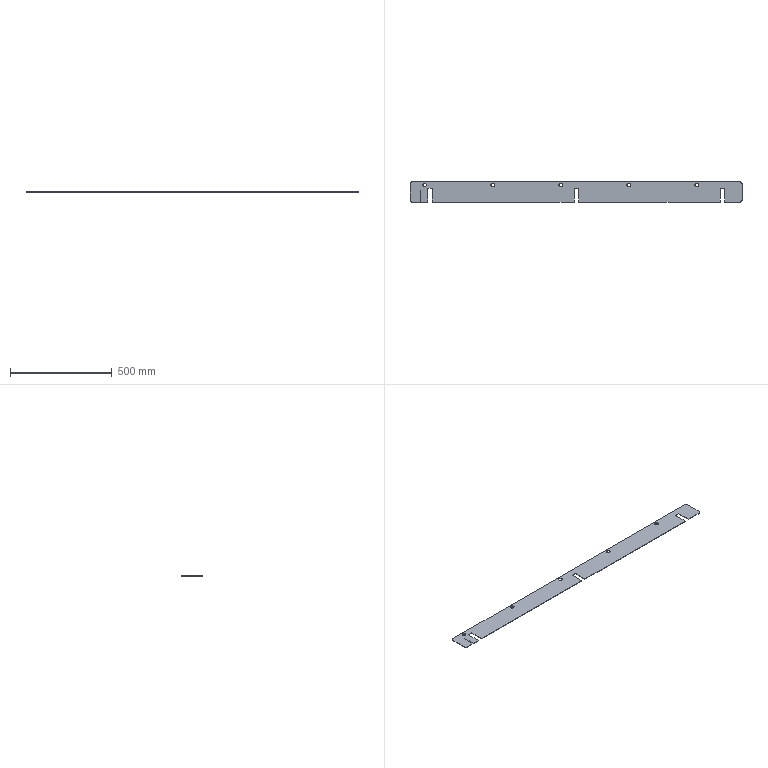Part | SolidWorks | features FlatPattern 1, SMBaseFlange 1, SheetMetal 1 | 1 solid | 36 faces | box 1635 x 100 x 2.3 mm | volume 362359 mm3 | plane 22 | cylinder 14 | commonest cylinder face diameters 18 x10 20 x4
STEP:
#1=CARTESIAN_POINT('',(398.,53.917,2.3));
#2=VERTEX_POINT('',#1);
#3=CARTESIAN_POINT('',(416.,53.917,2.3));
#4=VERTEX_POINT('',#3);
#5=CARTESIAN_POINT('',(407.,53.917,2.3));
#6=DIRECTION('',(0.,0.,1.));
#7=DIRECTION('',(1.,0.,0.));
#8=AXIS2_PLACEMENT_3D('',#5,#6,#7);
#9=CIRCLE('',#8,9.);
#10=EDGE_CURVE('',#2,#4,#9,.T.);
#11=ORIENTED_EDGE('',*,*,#10,.T.);
#12=CARTESIAN_POINT('',(416.,53.917,0.));
#13=VERTEX_POINT('',#12);
#14=CARTESIAN_POINT('',(416.,53.917,2.3));
#15=DIRECTION('',(0.,0.,-1.));
#16=VECTOR('',#15,1000.);
#17=LINE('',#14,#16);
#18=EDGE_CURVE('',#4,#13,#17,.T.);
#19=ORIENTED_EDGE('',*,*,#18,.T.);
#20=CARTESIAN_POINT('',(398.,53.917,0.));
#21=VERTEX_POINT('',#20);
#22=CARTESIAN_POINT('',(407.,53.917,0.));
#23=DIRECTION('',(0.,0.,1.));
#24=DIRECTION('',(1.,0.,0.));
#25=AXIS2_PLACEMENT_3D('',#22,#23,#24);
#26=CIRCLE('',#25,9.);
#27=EDGE_CURVE('',#21,#13,#26,.T.);
#28=ORIENTED_EDGE('',*,*,#27,.F.);
#29=CARTESIAN_POINT('',(398.,53.917,2.3));
#30=DIRECTION('',(0.,0.,-1.));
#31=VECTOR('',#30,1000.);
#32=LINE('',#29,#31);
#33=EDGE_CURVE('',#2,#21,#32,.T.);
#34=ORIENTED_EDGE('',*,*,#33,.F.);
#35=EDGE_LOOP('',(#11,#19,#28,#34));
#36=FACE_OUTER_BOUND('',#35,.T.);
#37=CARTESIAN_POINT('',(407.,53.917,2.3));
#38=DIRECTION('',(0.,0.,-1.));
#39=DIRECTION('',(-1.,0.,0.));
#40=AXIS2_PLACEMENT_3D('',#37,#38,#39);
#41=CYLINDRICAL_SURFACE('',#40,9.);
#42=ADVANCED_FACE('',(#36),#41,.F.);
#43=CARTESIAN_POINT('',(733.,53.917,2.3));
#44=VERTEX_POINT('',#43);
#45=CARTESIAN_POINT('',(751.,53.917,2.3));
#46=VERTEX_POINT('',#45);
#47=CARTESIAN_POINT('',(742.,53.917,2.3));
#48=DIRECTION('',(0.,0.,1.));
#49=DIRECTION('',(1.,0.,0.));
#50=AXIS2_PLACEMENT_3D('',#47,#48,#49);
#51=CIRCLE('',#50,9.);
#52=EDGE_CURVE('',#44,#46,#51,.T.);
#53=ORIENTED_EDGE('',*,*,#52,.T.);
#54=CARTESIAN_POINT('',(751.,53.917,0.));
#55=VERTEX_POINT('',#54);
#56=CARTESIAN_POINT('',(751.,53.917,2.3));
#57=DIRECTION('',(0.,0.,-1.));
#58=VECTOR('',#57,1000.);
#59=LINE('',#56,#58);
#60=EDGE_CURVE('',#46,#55,#59,.T.);
#61=ORIENTED_EDGE('',*,*,#60,.T.);
#62=CARTESIAN_POINT('',(733.,53.917,0.));
#63=VERTEX_POINT('',#62);
#64=CARTESIAN_POINT('',(742.,53.917,0.));
#65=DIRECTION('',(0.,0.,1.));
#66=DIRECTION('',(1.,0.,0.));
#67=AXIS2_PLACEMENT_3D('',#64,#65,#66);
#68=CIRCLE('',#67,9.);
#69=EDGE_CURVE('',#63,#55,#68,.T.);
#70=ORIENTED_EDGE('',*,*,#69,.F.);
#71=CARTESIAN_POINT('',(733.,53.917,2.3));
#72=DIRECTION('',(0.,0.,-1.));
#73=VECTOR('',#72,1000.);
#74=LINE('',#71,#73);
#75=EDGE_CURVE('',#44,#63,#74,.T.);
#76=ORIENTED_EDGE('',*,*,#75,.F.);
#77=EDGE_LOOP('',(#53,#61,#70,#76));
#78=FACE_OUTER_BOUND('',#77,.T.);
#79=CARTESIAN_POINT('',(742.,53.917,2.3));
#80=DIRECTION('',(0.,0.,-1.));
#81=DIRECTION('',(-1.,0.,0.));
#82=AXIS2_PLACEMENT_3D('',#79,#80,#81);
#83=CYLINDRICAL_SURFACE('',#82,9.);
#84=ADVANCED_FACE('',(#78),#83,.F.);
#85=CARTESIAN_POINT('',(1068.,53.917,2.3));
#86=VERTEX_POINT('',#85);
#87=CARTESIAN_POINT('',(1086.,53.917,2.3));
#88=VERTEX_POINT('',#87);
#89=CARTESIAN_POINT('',(1077.,53.917,2.3));
#90=DIRECTION('',(0.,0.,1.));
#91=DIRECTION('',(1.,0.,0.));
#92=AXIS2_PLACEMENT_3D('',#89,#90,#91);
#93=CIRCLE('',#92,9.);
#94=EDGE_CURVE('',#86,#88,#93,.T.);
#95=ORIENTED_EDGE('',*,*,#94,.T.);
#96=CARTESIAN_POINT('',(1086.,53.917,0.));
#97=VERTEX_POINT('',#96);
#98=CARTESIAN_POINT('',(1086.,53.917,2.3));
#99=DIRECTION('',(0.,0.,-1.));
#100=VECTOR('',#99,1000.);
#101=LINE('',#98,#100);
#102=EDGE_CURVE('',#88,#97,#101,.T.);
#103=ORIENTED_EDGE('',*,*,#102,.T.);
#104=CARTESIAN_POINT('',(1068.,53.917,0.));
#105=VERTEX_POINT('',#104);
#106=CARTESIAN_POINT('',(1077.,53.917,0.));
#107=DIRECTION('',(0.,0.,1.));
#108=DIRECTION('',(1.,0.,0.));
#109=AXIS2_PLACEMENT_3D('',#106,#107,#108);
#110=CIRCLE('',#109,9.);
#111=EDGE_CURVE('',#105,#97,#110,.T.);
#112=ORIENTED_EDGE('',*,*,#111,.F.);
#113=CARTESIAN_POINT('',(1068.,53.917,2.3));
#114=DIRECTION('',(0.,0.,-1.));
#115=VECTOR('',#114,1000.);
#116=LINE('',#113,#115);
#117=EDGE_CURVE('',#86,#105,#116,.T.);
#118=ORIENTED_EDGE('',*,*,#117,.F.);
#119=EDGE_LOOP('',(#95,#103,#112,#118));
#120=FACE_OUTER_BOUND('',#119,.T.);
#121=CARTESIAN_POINT('',(1077.,53.917,2.3));
#122=DIRECTION('',(0.,0.,-1.));
#123=DIRECTION('',(-1.,0.,0.));
#124=AXIS2_PLACEMENT_3D('',#121,#122,#123);
#125=CYLINDRICAL_SURFACE('',#124,9.);
#126=ADVANCED_FACE('',(#120),#125,.F.);
#127=CARTESIAN_POINT('',(63.,53.917,2.3));
#128=VERTEX_POINT('',#127);
#129=CARTESIAN_POINT('',(81.,53.917,2.3));
#130=VERTEX_POINT('',#129);
#131=CARTESIAN_POINT('',(72.,53.917,2.3));
#132=DIRECTION('',(0.,0.,1.));
#133=DIRECTION('',(1.,0.,0.));
#134=AXIS2_PLACEMENT_3D('',#131,#132,#133);
#135=CIRCLE('',#134,9.);
#136=EDGE_CURVE('',#128,#130,#135,.T.);
#137=ORIENTED_EDGE('',*,*,#136,.T.);
#138=CARTESIAN_POINT('',(81.,53.917,0.));
#139=VERTEX_POINT('',#138);
#140=CARTESIAN_POINT('',(81.,53.917,2.3));
#141=DIRECTION('',(0.,0.,-1.));
#142=VECTOR('',#141,1000.);
#143=LINE('',#140,#142);
#144=EDGE_CURVE('',#130,#139,#143,.T.);
#145=ORIENTED_EDGE('',*,*,#144,.T.);
#146=CARTESIAN_POINT('',(63.,53.917,0.));
#147=VERTEX_POINT('',#146);
#148=CARTESIAN_POINT('',(72.,53.917,0.));
#149=DIRECTION('',(0.,0.,1.));
#150=DIRECTION('',(1.,0.,0.));
#151=AXIS2_PLACEMENT_3D('',#148,#149,#150);
#152=CIRCLE('',#151,9.);
#153=EDGE_CURVE('',#147,#139,#152,.T.);
#154=ORIENTED_EDGE('',*,*,#153,.F.);
#155=CARTESIAN_POINT('',(63.,53.917,2.3));
#156=DIRECTION('',(0.,0.,-1.));
#157=VECTOR('',#156,1000.);
#158=LINE('',#155,#157);
#159=EDGE_CURVE('',#128,#147,#158,.T.);
#160=ORIENTED_EDGE('',*,*,#159,.F.);
#161=EDGE_LOOP('',(#137,#145,#154,#160));
#162=FACE_OUTER_BOUND('',#161,.T.);
#163=CARTESIAN_POINT('',(72.,53.917,2.3));
#164=DIRECTION('',(0.,0.,-1.));
#165=DIRECTION('',(-1.,0.,0.));
#166=AXIS2_PLACEMENT_3D('',#163,#164,#165);
#167=CYLINDRICAL_SURFACE('',#166,9.);
#168=ADVANCED_FACE('',(#162),#167,.F.);
#169=CARTESIAN_POINT('',(1403.,53.917,2.3));
#170=VERTEX_POINT('',#169);
#171=CARTESIAN_POINT('',(1421.,53.917,2.3));
#172=VERTEX_POINT('',#171);
#173=CARTESIAN_POINT('',(1412.,53.917,2.3));
#174=DIRECTION('',(0.,0.,1.));
#175=DIRECTION('',(1.,0.,0.));
#176=AXIS2_PLACEMENT_3D('',#173,#174,#175);
#177=CIRCLE('',#176,9.);
#178=EDGE_CURVE('',#170,#172,#177,.T.);
#179=ORIENTED_EDGE('',*,*,#178,.T.);
#180=CARTESIAN_POINT('',(1421.,53.917,0.));
#181=VERTEX_POINT('',#180);
#182=CARTESIAN_POINT('',(1421.,53.917,2.3));
#183=DIRECTION('',(0.,0.,-1.));
#184=VECTOR('',#183,1000.);
#185=LINE('',#182,#184);
#186=EDGE_CURVE('',#172,#181,#185,.T.);
#187=ORIENTED_EDGE('',*,*,#186,.T.);
#188=CARTESIAN_POINT('',(1403.,53.917,0.));
#189=VERTEX_POINT('',#188);
#190=CARTESIAN_POINT('',(1412.,53.917,0.));
#191=DIRECTION('',(0.,0.,1.));
#192=DIRECTION('',(1.,0.,0.));
#193=AXIS2_PLACEMENT_3D('',#190,#191,#192);
#194=CIRCLE('',#193,9.);
#195=EDGE_CURVE('',#189,#181,#194,.T.);
#196=ORIENTED_EDGE('',*,*,#195,.F.);
#197=CARTESIAN_POINT('',(1403.,53.917,2.3));
#198=DIRECTION('',(0.,0.,-1.));
#199=VECTOR('',#198,1000.);
#200=LINE('',#197,#199);
#201=EDGE_CURVE('',#170,#189,#200,.T.);
#202=ORIENTED_EDGE('',*,*,#201,.F.);
#203=EDGE_LOOP('',(#179,#187,#196,#202));
#204=FACE_OUTER_BOUND('',#203,.T.);
#205=CARTESIAN_POINT('',(1412.,53.917,2.3));
#206=DIRECTION('',(0.,0.,-1.));
#207=DIRECTION('',(-1.,0.,0.));
#208=AXIS2_PLACEMENT_3D('',#205,#206,#207);
#209=CYLINDRICAL_SURFACE('',#208,9.);
#210=ADVANCED_FACE('',(#204),#209,.F.);
#211=CARTESIAN_POINT('',(88.,38.092,2.3));
#212=VERTEX_POINT('',#211);
#213=CARTESIAN_POINT('',(110.,38.092,2.3));
#214=VERTEX_POINT('',#213);
#215=CARTESIAN_POINT('',(88.,38.092,2.3));
#216=DIRECTION('',(1.,0.,0.));
#217=VECTOR('',#216,1000.);
#218=LINE('',#215,#217);
#219=EDGE_CURVE('',#212,#214,#218,.T.);
#220=ORIENTED_EDGE('',*,*,#219,.T.);
#221=CARTESIAN_POINT('',(110.,-30.083,2.3));
#222=VERTEX_POINT('',#221);
#223=CARTESIAN_POINT('',(110.,38.092,2.3));
#224=DIRECTION('',(0.,-1.,0.));
#225=VECTOR('',#224,1000.);
#226=LINE('',#223,#225);
#227=EDGE_CURVE('',#214,#222,#226,.T.);
#228=ORIENTED_EDGE('',*,*,#227,.T.);
#229=CARTESIAN_POINT('',(808.,-30.083,2.3));
#230=VERTEX_POINT('',#229);
#231=CARTESIAN_POINT('',(110.,-30.083,2.3));
#232=DIRECTION('',(1.,0.,0.));
#233=VECTOR('',#232,1000.);
#234=LINE('',#231,#233);
#235=EDGE_CURVE('',#222,#230,#234,.T.);
#236=ORIENTED_EDGE('',*,*,#235,.T.);
#237=CARTESIAN_POINT('',(808.,38.092,2.3));
#238=VERTEX_POINT('',#237);
#239=CARTESIAN_POINT('',(808.,-30.083,2.3));
#240=DIRECTION('',(0.,1.,0.));
#241=VECTOR('',#240,1000.);
#242=LINE('',#239,#241);
#243=EDGE_CURVE('',#230,#238,#242,.T.);
#244=ORIENTED_EDGE('',*,*,#243,.T.);
#245=CARTESIAN_POINT('',(830.,38.092,2.3));
#246=VERTEX_POINT('',#245);
#247=CARTESIAN_POINT('',(808.,38.092,2.3));
#248=DIRECTION('',(1.,0.,0.));
#249=VECTOR('',#248,1000.);
#250=LINE('',#247,#249);
#251=EDGE_CURVE('',#238,#246,#250,.T.);
#252=ORIENTED_EDGE('',*,*,#251,.T.);
#253=CARTESIAN_POINT('',(830.,-30.083,2.3));
#254=VERTEX_POINT('',#253);
#255=CARTESIAN_POINT('',(830.,38.092,2.3));
#256=DIRECTION('',(0.,-1.,0.));
#257=VECTOR('',#256,1000.);
#258=LINE('',#255,#257);
#259=EDGE_CURVE('',#246,#254,#258,.T.);
#260=ORIENTED_EDGE('',*,*,#259,.T.);
#261=CARTESIAN_POINT('',(1528.,-30.083,2.3));
#262=VERTEX_POINT('',#261);
#263=CARTESIAN_POINT('',(830.,-30.083,2.3));
#264=DIRECTION('',(1.,0.,0.));
#265=VECTOR('',#264,1000.);
#266=LINE('',#263,#265);
#267=EDGE_CURVE('',#254,#262,#266,.T.);
#268=ORIENTED_EDGE('',*,*,#267,.T.);
#269=CARTESIAN_POINT('',(1528.,38.092,2.3));
#270=VERTEX_POINT('',#269);
#271=CARTESIAN_POINT('',(1528.,-30.083,2.3));
#272=DIRECTION('',(0.,1.,0.));
#273=VECTOR('',#272,1000.);
#274=LINE('',#271,#273);
#275=EDGE_CURVE('',#262,#270,#274,.T.);
#276=ORIENTED_EDGE('',*,*,#275,.T.);
#277=CARTESIAN_POINT('',(1550.,38.092,2.3));
#278=VERTEX_POINT('',#277);
#279=CARTESIAN_POINT('',(1528.,38.092,2.3));
#280=DIRECTION('',(1.,0.,0.));
#281=VECTOR('',#280,1000.);
#282=LINE('',#279,#281);
#283=EDGE_CURVE('',#270,#278,#282,.T.);
#284=ORIENTED_EDGE('',*,*,#283,.T.);
#285=CARTESIAN_POINT('',(1550.,-30.083,2.3));
#286=VERTEX_POINT('',#285);
#287=CARTESIAN_POINT('',(1550.,38.092,2.3));
#288=DIRECTION('',(0.,-1.,0.));
#289=VECTOR('',#288,1000.);
#290=LINE('',#287,#289);
#291=EDGE_CURVE('',#278,#286,#290,.T.);
#292=ORIENTED_EDGE('',*,*,#291,.T.);
#293=CARTESIAN_POINT('',(1625.,-30.083,2.3));
#294=VERTEX_POINT('',#293);
#295=CARTESIAN_POINT('',(1550.,-30.083,2.3));
#296=DIRECTION('',(1.,0.,0.));
#297=VECTOR('',#296,1000.);
#298=LINE('',#295,#297);
#299=EDGE_CURVE('',#286,#294,#298,.T.);
#300=ORIENTED_EDGE('',*,*,#299,.T.);
#301=CARTESIAN_POINT('',(1635.,-20.083,2.3));
#302=VERTEX_POINT('',#301);
#303=CARTESIAN_POINT('',(1625.,-20.083,2.3));
#304=DIRECTION('',(0.,0.,1.));
#305=DIRECTION('',(-1.,0.,0.));
#306=AXIS2_PLACEMENT_3D('',#303,#304,#305);
#307=CIRCLE('',#306,10.);
#308=EDGE_CURVE('',#294,#302,#307,.T.);
#309=ORIENTED_EDGE('',*,*,#308,.T.);
#310=CARTESIAN_POINT('',(1635.,59.917,2.3));
#311=VERTEX_POINT('',#310);
#312=CARTESIAN_POINT('',(1635.,-20.083,2.3));
#313=DIRECTION('',(0.,1.,0.));
#314=VECTOR('',#313,1000.);
#315=LINE('',#312,#314);
#316=EDGE_CURVE('',#302,#311,#315,.T.);
#317=ORIENTED_EDGE('',*,*,#316,.T.);
#318=CARTESIAN_POINT('',(1625.,69.917,2.3));
#319=VERTEX_POINT('',#318);
#320=CARTESIAN_POINT('',(1625.,59.917,2.3));
#321=DIRECTION('',(0.,0.,1.));
#322=DIRECTION('',(1.,0.,0.));
#323=AXIS2_PLACEMENT_3D('',#320,#321,#322);
#324=CIRCLE('',#323,10.);
#325=EDGE_CURVE('',#311,#319,#324,.T.);
#326=ORIENTED_EDGE('',*,*,#325,.T.);
#327=CARTESIAN_POINT('',(10.,69.917,2.3));
#328=VERTEX_POINT('',#327);
#329=CARTESIAN_POINT('',(1625.,69.917,2.3));
#330=DIRECTION('',(-1.,0.,0.));
#331=VECTOR('',#330,1000.);
#332=LINE('',#329,#331);
#333=EDGE_CURVE('',#319,#328,#332,.T.);
#334=ORIENTED_EDGE('',*,*,#333,.T.);
#335=CARTESIAN_POINT('',(0.,59.917,2.3));
#336=VERTEX_POINT('',#335);
#337=CARTESIAN_POINT('',(10.,59.917,2.3));
#338=DIRECTION('',(0.,0.,1.));
#339=DIRECTION('',(1.,0.,0.));
#340=AXIS2_PLACEMENT_3D('',#337,#338,#339);
#341=CIRCLE('',#340,10.);
#342=EDGE_CURVE('',#328,#336,#341,.T.);
#343=ORIENTED_EDGE('',*,*,#342,.T.);
#344=CARTESIAN_POINT('',(0.,-20.083,2.3));
#345=VERTEX_POINT('',#344);
#346=CARTESIAN_POINT('',(0.,59.917,2.3));
#347=DIRECTION('',(0.,-1.,0.));
#348=VECTOR('',#347,1000.);
#349=LINE('',#346,#348);
#350=EDGE_CURVE('',#336,#345,#349,.T.);
#351=ORIENTED_EDGE('',*,*,#350,.T.);
#352=CARTESIAN_POINT('',(10.,-30.083,2.3));
#353=VERTEX_POINT('',#352);
#354=CARTESIAN_POINT('',(10.,-20.083,2.3));
#355=DIRECTION('',(0.,0.,1.));
#356=DIRECTION('',(1.,0.,0.));
#357=AXIS2_PLACEMENT_3D('',#354,#355,#356);
#358=CIRCLE('',#357,10.);
#359=EDGE_CURVE('',#345,#353,#358,.T.);
#360=ORIENTED_EDGE('',*,*,#359,.T.);
#361=CARTESIAN_POINT('',(50.4,-30.083,2.3));
#362=VERTEX_POINT('',#361);
#363=CARTESIAN_POINT('',(10.,-30.083,2.3));
#364=DIRECTION('',(1.,0.,0.));
#365=VECTOR('',#364,1000.);
#366=LINE('',#363,#365);
#367=EDGE_CURVE('',#353,#362,#366,.T.);
#368=ORIENTED_EDGE('',*,*,#367,.T.);
#369=CARTESIAN_POINT('',(50.4,29.082,2.3));
#370=VERTEX_POINT('',#369);
#371=CARTESIAN_POINT('',(50.4,29.082,2.3));
#372=DIRECTION('',(0.,1.,0.));
#373=VECTOR('',#372,1000.);
#374=LINE('',#371,#373);
#375=EDGE_CURVE('',#362,#370,#374,.T.);
#376=ORIENTED_EDGE('',*,*,#375,.T.);
#377=CARTESIAN_POINT('',(52.,29.082,2.3));
#378=VERTEX_POINT('',#377);
#379=CARTESIAN_POINT('',(52.,29.082,2.3));
#380=DIRECTION('',(1.,0.,0.));
#381=VECTOR('',#380,1000.);
#382=LINE('',#379,#381);
#383=EDGE_CURVE('',#370,#378,#382,.T.);
#384=ORIENTED_EDGE('',*,*,#383,.T.);
#385=CARTESIAN_POINT('',(52.,-30.083,2.3));
#386=VERTEX_POINT('',#385);
#387=CARTESIAN_POINT('',(52.,-30.083,2.3));
#388=DIRECTION('',(0.,-1.,0.));
#389=VECTOR('',#388,1000.);
#390=LINE('',#387,#389);
#391=EDGE_CURVE('',#378,#386,#390,.T.);
#392=ORIENTED_EDGE('',*,*,#391,.T.);
#393=CARTESIAN_POINT('',(88.,-30.083,2.3));
#394=VERTEX_POINT('',#393);
#395=CARTESIAN_POINT('',(52.,-30.083,2.3));
#396=DIRECTION('',(1.,0.,0.));
#397=VECTOR('',#396,1000.);
#398=LINE('',#395,#397);
#399=EDGE_CURVE('',#386,#394,#398,.T.);
#400=ORIENTED_EDGE('',*,*,#399,.T.);
#401=CARTESIAN_POINT('',(88.,-30.083,2.3));
#402=DIRECTION('',(0.,1.,0.));
#403=VECTOR('',#402,1000.);
#404=LINE('',#401,#403);
#405=EDGE_CURVE('',#394,#212,#404,.T.);
#406=ORIENTED_EDGE('',*,*,#405,.T.);
#407=EDGE_LOOP('',(#220,#228,#236,#244,#252,#260,#268,#276,#284,#292,#300,#309,#317,#326,#334,#343,#351,#360,#368,#376,#384,#392,#400,#406));
#408=FACE_OUTER_BOUND('',#407,.T.);
#409=ORIENTED_EDGE('',*,*,#178,.F.);
#410=CARTESIAN_POINT('',(1412.,53.917,2.3));
#411=DIRECTION('',(0.,0.,1.));
#412=DIRECTION('',(1.,0.,0.));
#413=AXIS2_PLACEMENT_3D('',#410,#411,#412);
#414=CIRCLE('',#413,9.);
#415=EDGE_CURVE('',#172,#170,#414,.T.);
#416=ORIENTED_EDGE('',*,*,#415,.F.);
#417=EDGE_LOOP('',(#409,#416));
#418=FACE_BOUND('',#417,.T.);
#419=ORIENTED_EDGE('',*,*,#136,.F.);
#420=CARTESIAN_POINT('',(72.,53.917,2.3));
#421=DIRECTION('',(0.,0.,1.));
#422=DIRECTION('',(1.,0.,0.));
#423=AXIS2_PLACEMENT_3D('',#420,#421,#422);
#424=CIRCLE('',#423,9.);
#425=EDGE_CURVE('',#130,#128,#424,.T.);
#426=ORIENTED_EDGE('',*,*,#425,.F.);
#427=EDGE_LOOP('',(#419,#426));
#428=FACE_BOUND('',#427,.T.);
#429=ORIENTED_EDGE('',*,*,#94,.F.);
#430=CARTESIAN_POINT('',(1077.,53.917,2.3));
#431=DIRECTION('',(0.,0.,1.));
#432=DIRECTION('',(1.,0.,0.));
#433=AXIS2_PLACEMENT_3D('',#430,#431,#432);
#434=CIRCLE('',#433,9.);
#435=EDGE_CURVE('',#88,#86,#434,.T.);
#436=ORIENTED_EDGE('',*,*,#435,.F.);
#437=EDGE_LOOP('',(#429,#436));
#438=FACE_BOUND('',#437,.T.);
#439=ORIENTED_EDGE('',*,*,#52,.F.);
#440=CARTESIAN_POINT('',(742.,53.917,2.3));
#441=DIRECTION('',(0.,0.,1.));
#442=DIRECTION('',(1.,0.,0.));
#443=AXIS2_PLACEMENT_3D('',#440,#441,#442);
#444=CIRCLE('',#443,9.);
#445=EDGE_CURVE('',#46,#44,#444,.T.);
#446=ORIENTED_EDGE('',*,*,#445,.F.);
#447=EDGE_LOOP('',(#439,#446));
#448=FACE_BOUND('',#447,.T.);
#449=ORIENTED_EDGE('',*,*,#10,.F.);
#450=CARTESIAN_POINT('',(407.,53.917,2.3));
#451=DIRECTION('',(0.,0.,1.));
#452=DIRECTION('',(1.,0.,0.));
#453=AXIS2_PLACEMENT_3D('',#450,#451,#452);
#454=CIRCLE('',#453,9.);
#455=EDGE_CURVE('',#4,#2,#454,.T.);
#456=ORIENTED_EDGE('',*,*,#455,.F.);
#457=EDGE_LOOP('',(#449,#456));
#458=FACE_BOUND('',#457,.T.);
#459=CARTESIAN_POINT('',(1625.,-20.083,2.3));
#460=DIRECTION('',(0.,0.,-1.));
#461=DIRECTION('',(-1.,0.,0.));
#462=AXIS2_PLACEMENT_3D('',#459,#460,#461);
#463=PLANE('',#462);
#464=ADVANCED_FACE('',(#408,#418,#428,#438,#448,#458),#463,.F.);
#465=ORIENTED_EDGE('',*,*,#69,.T.);
#466=CARTESIAN_POINT('',(742.,53.917,0.));
#467=DIRECTION('',(0.,0.,1.));
#468=DIRECTION('',(1.,0.,0.));
#469=AXIS2_PLACEMENT_3D('',#466,#467,#468);
#470=CIRCLE('',#469,9.);
#471=EDGE_CURVE('',#55,#63,#470,.T.);
#472=ORIENTED_EDGE('',*,*,#471,.T.);
#473=EDGE_LOOP('',(#465,#472));
#474=FACE_BOUND('',#473,.T.);
#475=ORIENTED_EDGE('',*,*,#153,.T.);
#476=CARTESIAN_POINT('',(72.,53.917,0.));
#477=DIRECTION('',(0.,0.,1.));
#478=DIRECTION('',(1.,0.,0.));
#479=AXIS2_PLACEMENT_3D('',#476,#477,#478);
#480=CIRCLE('',#479,9.);
#481=EDGE_CURVE('',#139,#147,#480,.T.);
#482=ORIENTED_EDGE('',*,*,#481,.T.);
#483=EDGE_LOOP('',(#475,#482));
#484=FACE_BOUND('',#483,.T.);
#485=CARTESIAN_POINT('',(88.,38.092,0.));
#486=VERTEX_POINT('',#485);
#487=CARTESIAN_POINT('',(110.,38.092,0.));
#488=VERTEX_POINT('',#487);
#489=CARTESIAN_POINT('',(88.,38.092,0.));
#490=DIRECTION('',(1.,0.,0.));
#491=VECTOR('',#490,1000.);
#492=LINE('',#489,#491);
#493=EDGE_CURVE('',#486,#488,#492,.T.);
#494=ORIENTED_EDGE('',*,*,#493,.F.);
#495=CARTESIAN_POINT('',(88.,-30.083,0.));
#496=VERTEX_POINT('',#495);
#497=CARTESIAN_POINT('',(88.,-30.083,0.));
#498=DIRECTION('',(0.,1.,0.));
#499=VECTOR('',#498,1000.);
#500=LINE('',#497,#499);
#501=EDGE_CURVE('',#496,#486,#500,.T.);
#502=ORIENTED_EDGE('',*,*,#501,.F.);
#503=CARTESIAN_POINT('',(52.,-30.083,0.));
#504=VERTEX_POINT('',#503);
#505=CARTESIAN_POINT('',(52.,-30.083,0.));
#506=DIRECTION('',(1.,0.,0.));
#507=VECTOR('',#506,1000.);
#508=LINE('',#505,#507);
#509=EDGE_CURVE('',#504,#496,#508,.T.);
#510=ORIENTED_EDGE('',*,*,#509,.F.);
#511=CARTESIAN_POINT('',(52.,29.082,0.));
#512=VERTEX_POINT('',#511);
#513=CARTESIAN_POINT('',(52.,-30.083,0.));
#514=DIRECTION('',(0.,-1.,0.));
#515=VECTOR('',#514,1000.);
#516=LINE('',#513,#515);
#517=EDGE_CURVE('',#512,#504,#516,.T.);
#518=ORIENTED_EDGE('',*,*,#517,.F.);
#519=CARTESIAN_POINT('',(50.4,29.082,0.));
#520=VERTEX_POINT('',#519);
#521=CARTESIAN_POINT('',(52.,29.082,0.));
#522=DIRECTION('',(1.,0.,0.));
#523=VECTOR('',#522,1000.);
#524=LINE('',#521,#523);
#525=EDGE_CURVE('',#520,#512,#524,.T.);
#526=ORIENTED_EDGE('',*,*,#525,.F.);
#527=CARTESIAN_POINT('',(50.4,-30.083,0.));
#528=VERTEX_POINT('',#527);
#529=CARTESIAN_POINT('',(50.4,29.082,0.));
#530=DIRECTION('',(0.,1.,0.));
#531=VECTOR('',#530,1000.);
#532=LINE('',#529,#531);
#533=EDGE_CURVE('',#528,#520,#532,.T.);
#534=ORIENTED_EDGE('',*,*,#533,.F.);
#535=CARTESIAN_POINT('',(10.,-30.083,0.));
#536=VERTEX_POINT('',#535);
#537=CARTESIAN_POINT('',(10.,-30.083,0.));
#538=DIRECTION('',(1.,0.,0.));
#539=VECTOR('',#538,1000.);
#540=LINE('',#537,#539);
#541=EDGE_CURVE('',#536,#528,#540,.T.);
#542=ORIENTED_EDGE('',*,*,#541,.F.);
#543=CARTESIAN_POINT('',(0.,-20.083,0.));
#544=VERTEX_POINT('',#543);
#545=CARTESIAN_POINT('',(10.,-20.083,0.));
#546=DIRECTION('',(0.,0.,1.));
#547=DIRECTION('',(1.,0.,0.));
#548=AXIS2_PLACEMENT_3D('',#545,#546,#547);
#549=CIRCLE('',#548,10.);
#550=EDGE_CURVE('',#544,#536,#549,.T.);
#551=ORIENTED_EDGE('',*,*,#550,.F.);
#552=CARTESIAN_POINT('',(0.,59.917,0.));
#553=VERTEX_POINT('',#552);
#554=CARTESIAN_POINT('',(0.,59.917,0.));
#555=DIRECTION('',(0.,-1.,0.));
#556=VECTOR('',#555,1000.);
#557=LINE('',#554,#556);
#558=EDGE_CURVE('',#553,#544,#557,.T.);
#559=ORIENTED_EDGE('',*,*,#558,.F.);
#560=CARTESIAN_POINT('',(10.,69.917,0.));
#561=VERTEX_POINT('',#560);
#562=CARTESIAN_POINT('',(10.,59.917,0.));
#563=DIRECTION('',(0.,0.,1.));
#564=DIRECTION('',(1.,0.,0.));
#565=AXIS2_PLACEMENT_3D('',#562,#563,#564);
#566=CIRCLE('',#565,10.);
#567=EDGE_CURVE('',#561,#553,#566,.T.);
#568=ORIENTED_EDGE('',*,*,#567,.F.);
#569=CARTESIAN_POINT('',(1625.,69.917,0.));
#570=VERTEX_POINT('',#569);
#571=CARTESIAN_POINT('',(1625.,69.917,0.));
#572=DIRECTION('',(-1.,0.,0.));
#573=VECTOR('',#572,1000.);
#574=LINE('',#571,#573);
#575=EDGE_CURVE('',#570,#561,#574,.T.);
#576=ORIENTED_EDGE('',*,*,#575,.F.);
#577=CARTESIAN_POINT('',(1635.,59.917,0.));
#578=VERTEX_POINT('',#577);
#579=CARTESIAN_POINT('',(1625.,59.917,0.));
#580=DIRECTION('',(0.,0.,1.));
#581=DIRECTION('',(1.,0.,0.));
#582=AXIS2_PLACEMENT_3D('',#579,#580,#581);
#583=CIRCLE('',#582,10.);
#584=EDGE_CURVE('',#578,#570,#583,.T.);
#585=ORIENTED_EDGE('',*,*,#584,.F.);
#586=CARTESIAN_POINT('',(1635.,-20.083,0.));
#587=VERTEX_POINT('',#586);
#588=CARTESIAN_POINT('',(1635.,-20.083,0.));
#589=DIRECTION('',(0.,1.,0.));
#590=VECTOR('',#589,1000.);
#591=LINE('',#588,#590);
#592=EDGE_CURVE('',#587,#578,#591,.T.);
#593=ORIENTED_EDGE('',*,*,#592,.F.);
#594=CARTESIAN_POINT('',(1625.,-30.083,0.));
#595=VERTEX_POINT('',#594);
#596=CARTESIAN_POINT('',(1625.,-20.083,0.));
#597=DIRECTION('',(0.,0.,1.));
#598=DIRECTION('',(-1.,0.,0.));
#599=AXIS2_PLACEMENT_3D('',#596,#597,#598);
#600=CIRCLE('',#599,10.);
#601=EDGE_CURVE('',#595,#587,#600,.T.);
#602=ORIENTED_EDGE('',*,*,#601,.F.);
#603=CARTESIAN_POINT('',(1550.,-30.083,0.));
#604=VERTEX_POINT('',#603);
#605=CARTESIAN_POINT('',(1550.,-30.083,0.));
#606=DIRECTION('',(1.,0.,0.));
#607=VECTOR('',#606,1000.);
#608=LINE('',#605,#607);
#609=EDGE_CURVE('',#604,#595,#608,.T.);
#610=ORIENTED_EDGE('',*,*,#609,.F.);
#611=CARTESIAN_POINT('',(1550.,38.092,0.));
#612=VERTEX_POINT('',#611);
#613=CARTESIAN_POINT('',(1550.,38.092,0.));
#614=DIRECTION('',(0.,-1.,0.));
#615=VECTOR('',#614,1000.);
#616=LINE('',#613,#615);
#617=EDGE_CURVE('',#612,#604,#616,.T.);
#618=ORIENTED_EDGE('',*,*,#617,.F.);
#619=CARTESIAN_POINT('',(1528.,38.092,0.));
#620=VERTEX_POINT('',#619);
#621=CARTESIAN_POINT('',(1528.,38.092,0.));
#622=DIRECTION('',(1.,0.,0.));
#623=VECTOR('',#622,1000.);
#624=LINE('',#621,#623);
#625=EDGE_CURVE('',#620,#612,#624,.T.);
#626=ORIENTED_EDGE('',*,*,#625,.F.);
#627=CARTESIAN_POINT('',(1528.,-30.083,0.));
#628=VERTEX_POINT('',#627);
#629=CARTESIAN_POINT('',(1528.,-30.083,0.));
#630=DIRECTION('',(0.,1.,0.));
#631=VECTOR('',#630,1000.);
#632=LINE('',#629,#631);
#633=EDGE_CURVE('',#628,#620,#632,.T.);
#634=ORIENTED_EDGE('',*,*,#633,.F.);
#635=CARTESIAN_POINT('',(830.,-30.083,0.));
#636=VERTEX_POINT('',#635);
#637=CARTESIAN_POINT('',(830.,-30.083,0.));
#638=DIRECTION('',(1.,0.,0.));
#639=VECTOR('',#638,1000.);
#640=LINE('',#637,#639);
#641=EDGE_CURVE('',#636,#628,#640,.T.);
#642=ORIENTED_EDGE('',*,*,#641,.F.);
#643=CARTESIAN_POINT('',(830.,38.092,0.));
#644=VERTEX_POINT('',#643);
#645=CARTESIAN_POINT('',(830.,38.092,0.));
#646=DIRECTION('',(0.,-1.,0.));
#647=VECTOR('',#646,1000.);
#648=LINE('',#645,#647);
#649=EDGE_CURVE('',#644,#636,#648,.T.);
#650=ORIENTED_EDGE('',*,*,#649,.F.);
#651=CARTESIAN_POINT('',(808.,38.092,0.));
#652=VERTEX_POINT('',#651);
#653=CARTESIAN_POINT('',(808.,38.092,0.));
#654=DIRECTION('',(1.,0.,0.));
#655=VECTOR('',#654,1000.);
#656=LINE('',#653,#655);
#657=EDGE_CURVE('',#652,#644,#656,.T.);
#658=ORIENTED_EDGE('',*,*,#657,.F.);
#659=CARTESIAN_POINT('',(808.,-30.083,0.));
#660=VERTEX_POINT('',#659);
#661=CARTESIAN_POINT('',(808.,-30.083,0.));
#662=DIRECTION('',(0.,1.,0.));
#663=VECTOR('',#662,1000.);
#664=LINE('',#661,#663);
#665=EDGE_CURVE('',#660,#652,#664,.T.);
#666=ORIENTED_EDGE('',*,*,#665,.F.);
#667=CARTESIAN_POINT('',(110.,-30.083,0.));
#668=VERTEX_POINT('',#667);
#669=CARTESIAN_POINT('',(110.,-30.083,0.));
#670=DIRECTION('',(1.,0.,0.));
#671=VECTOR('',#670,1000.);
#672=LINE('',#669,#671);
#673=EDGE_CURVE('',#668,#660,#672,.T.);
#674=ORIENTED_EDGE('',*,*,#673,.F.);
#675=CARTESIAN_POINT('',(110.,38.092,0.));
#676=DIRECTION('',(0.,-1.,0.));
#677=VECTOR('',#676,1000.);
#678=LINE('',#675,#677);
#679=EDGE_CURVE('',#488,#668,#678,.T.);
#680=ORIENTED_EDGE('',*,*,#679,.F.);
#681=EDGE_LOOP('',(#494,#502,#510,#518,#526,#534,#542,#551,#559,#568,#576,#585,#593,#602,#610,#618,#626,#634,#642,#650,#658,#666,#674,#680));
#682=FACE_OUTER_BOUND('',#681,.T.);
#683=ORIENTED_EDGE('',*,*,#195,.T.);
#684=CARTESIAN_POINT('',(1412.,53.917,0.));
#685=DIRECTION('',(0.,0.,1.));
#686=DIRECTION('',(1.,0.,0.));
#687=AXIS2_PLACEMENT_3D('',#684,#685,#686);
#688=CIRCLE('',#687,9.);
#689=EDGE_CURVE('',#181,#189,#688,.T.);
#690=ORIENTED_EDGE('',*,*,#689,.T.);
#691=EDGE_LOOP('',(#683,#690));
#692=FACE_BOUND('',#691,.T.);
#693=ORIENTED_EDGE('',*,*,#111,.T.);
#694=CARTESIAN_POINT('',(1077.,53.917,0.));
#695=DIRECTION('',(0.,0.,1.));
#696=DIRECTION('',(1.,0.,0.));
#697=AXIS2_PLACEMENT_3D('',#694,#695,#696);
#698=CIRCLE('',#697,9.);
#699=EDGE_CURVE('',#97,#105,#698,.T.);
#700=ORIENTED_EDGE('',*,*,#699,.T.);
#701=EDGE_LOOP('',(#693,#700));
#702=FACE_BOUND('',#701,.T.);
#703=ORIENTED_EDGE('',*,*,#27,.T.);
#704=CARTESIAN_POINT('',(407.,53.917,0.));
#705=DIRECTION('',(0.,0.,1.));
#706=DIRECTION('',(1.,0.,0.));
#707=AXIS2_PLACEMENT_3D('',#704,#705,#706);
#708=CIRCLE('',#707,9.);
#709=EDGE_CURVE('',#13,#21,#708,.T.);
#710=ORIENTED_EDGE('',*,*,#709,.T.);
#711=EDGE_LOOP('',(#703,#710));
#712=FACE_BOUND('',#711,.T.);
#713=CARTESIAN_POINT('',(1625.,-20.083,0.));
#714=DIRECTION('',(0.,0.,-1.));
#715=DIRECTION('',(-1.,0.,0.));
#716=AXIS2_PLACEMENT_3D('',#713,#714,#715);
#717=PLANE('',#716);
#718=ADVANCED_FACE('',(#474,#484,#682,#692,#702,#712),#717,.T.);
#719=ORIENTED_EDGE('',*,*,#493,.T.);
#720=CARTESIAN_POINT('',(110.,38.092,2.3));
#721=DIRECTION('',(0.,0.,-1.));
#722=VECTOR('',#721,1000.);
#723=LINE('',#720,#722);
#724=EDGE_CURVE('',#214,#488,#723,.T.);
#725=ORIENTED_EDGE('',*,*,#724,.F.);
#726=ORIENTED_EDGE('',*,*,#219,.F.);
#727=CARTESIAN_POINT('',(88.,38.092,2.3));
#728=DIRECTION('',(0.,0.,-1.));
#729=VECTOR('',#728,1000.);
#730=LINE('',#727,#729);
#731=EDGE_CURVE('',#212,#486,#730,.T.);
#732=ORIENTED_EDGE('',*,*,#731,.T.);
#733=EDGE_LOOP('',(#719,#725,#726,#732));
#734=FACE_OUTER_BOUND('',#733,.T.);
#735=CARTESIAN_POINT('',(88.,38.092,2.3));
#736=DIRECTION('',(0.,1.,0.));
#737=DIRECTION('',(0.,0.,1.));
#738=AXIS2_PLACEMENT_3D('',#735,#736,#737);
#739=PLANE('',#738);
#740=ADVANCED_FACE('',(#734),#739,.F.);
#741=ORIENTED_EDGE('',*,*,#679,.T.);
#742=CARTESIAN_POINT('',(110.,-30.083,2.3));
#743=DIRECTION('',(0.,0.,-1.));
#744=VECTOR('',#743,1000.);
#745=LINE('',#742,#744);
#746=EDGE_CURVE('',#222,#668,#745,.T.);
#747=ORIENTED_EDGE('',*,*,#746,.F.);
#748=ORIENTED_EDGE('',*,*,#227,.F.);
#749=ORIENTED_EDGE('',*,*,#724,.T.);
#750=EDGE_LOOP('',(#741,#747,#748,#749));
#751=FACE_OUTER_BOUND('',#750,.T.);
#752=CARTESIAN_POINT('',(110.,38.092,2.3));
#753=DIRECTION('',(1.,0.,0.));
#754=DIRECTION('',(0.,1.,0.));
#755=AXIS2_PLACEMENT_3D('',#752,#753,#754);
#756=PLANE('',#755);
#757=ADVANCED_FACE('',(#751),#756,.F.);
#758=ORIENTED_EDGE('',*,*,#673,.T.);
#759=CARTESIAN_POINT('',(808.,-30.083,2.3));
#760=DIRECTION('',(0.,0.,-1.));
#761=VECTOR('',#760,1000.);
#762=LINE('',#759,#761);
#763=EDGE_CURVE('',#230,#660,#762,.T.);
#764=ORIENTED_EDGE('',*,*,#763,.F.);
#765=ORIENTED_EDGE('',*,*,#235,.F.);
#766=ORIENTED_EDGE('',*,*,#746,.T.);
#767=EDGE_LOOP('',(#758,#764,#765,#766));
#768=FACE_OUTER_BOUND('',#767,.T.);
#769=CARTESIAN_POINT('',(110.,-30.083,2.3));
#770=DIRECTION('',(0.,1.,0.));
#771=DIRECTION('',(0.,0.,1.));
#772=AXIS2_PLACEMENT_3D('',#769,#770,#771);
#773=PLANE('',#772);
#774=ADVANCED_FACE('',(#768),#773,.F.);
#775=ORIENTED_EDGE('',*,*,#665,.T.);
#776=CARTESIAN_POINT('',(808.,38.092,2.3));
#777=DIRECTION('',(0.,0.,-1.));
#778=VECTOR('',#777,1000.);
#779=LINE('',#776,#778);
#780=EDGE_CURVE('',#238,#652,#779,.T.);
#781=ORIENTED_EDGE('',*,*,#780,.F.);
#782=ORIENTED_EDGE('',*,*,#243,.F.);
#783=ORIENTED_EDGE('',*,*,#763,.T.);
#784=EDGE_LOOP('',(#775,#781,#782,#783));
#785=FACE_OUTER_BOUND('',#784,.T.);
#786=CARTESIAN_POINT('',(808.,-30.083,2.3));
#787=DIRECTION('',(-1.,0.,0.));
#788=DIRECTION('',(0.,0.,1.));
#789=AXIS2_PLACEMENT_3D('',#786,#787,#788);
#790=PLANE('',#789);
#791=ADVANCED_FACE('',(#785),#790,.F.);
#792=ORIENTED_EDGE('',*,*,#657,.T.);
#793=CARTESIAN_POINT('',(830.,38.092,2.3));
#794=DIRECTION('',(0.,0.,-1.));
#795=VECTOR('',#794,1000.);
#796=LINE('',#793,#795);
#797=EDGE_CURVE('',#246,#644,#796,.T.);
#798=ORIENTED_EDGE('',*,*,#797,.F.);
#799=ORIENTED_EDGE('',*,*,#251,.F.);
#800=ORIENTED_EDGE('',*,*,#780,.T.);
#801=EDGE_LOOP('',(#792,#798,#799,#800));
#802=FACE_OUTER_BOUND('',#801,.T.);
#803=CARTESIAN_POINT('',(808.,38.092,2.3));
#804=DIRECTION('',(0.,1.,0.));
#805=DIRECTION('',(0.,0.,1.));
#806=AXIS2_PLACEMENT_3D('',#803,#804,#805);
#807=PLANE('',#806);
#808=ADVANCED_FACE('',(#802),#807,.F.);
#809=ORIENTED_EDGE('',*,*,#649,.T.);
#810=CARTESIAN_POINT('',(830.,-30.083,2.3));
#811=DIRECTION('',(0.,0.,-1.));
#812=VECTOR('',#811,1000.);
#813=LINE('',#810,#812);
#814=EDGE_CURVE('',#254,#636,#813,.T.);
#815=ORIENTED_EDGE('',*,*,#814,.F.);
#816=ORIENTED_EDGE('',*,*,#259,.F.);
#817=ORIENTED_EDGE('',*,*,#797,.T.);
#818=EDGE_LOOP('',(#809,#815,#816,#817));
#819=FACE_OUTER_BOUND('',#818,.T.);
#820=CARTESIAN_POINT('',(830.,38.092,2.3));
#821=DIRECTION('',(1.,0.,0.));
#822=DIRECTION('',(0.,0.,-1.));
#823=AXIS2_PLACEMENT_3D('',#820,#821,#822);
#824=PLANE('',#823);
#825=ADVANCED_FACE('',(#819),#824,.F.);
#826=ORIENTED_EDGE('',*,*,#641,.T.);
#827=CARTESIAN_POINT('',(1528.,-30.083,2.3));
#828=DIRECTION('',(0.,0.,-1.));
#829=VECTOR('',#828,1000.);
#830=LINE('',#827,#829);
#831=EDGE_CURVE('',#262,#628,#830,.T.);
#832=ORIENTED_EDGE('',*,*,#831,.F.);
#833=ORIENTED_EDGE('',*,*,#267,.F.);
#834=ORIENTED_EDGE('',*,*,#814,.T.);
#835=EDGE_LOOP('',(#826,#832,#833,#834));
#836=FACE_OUTER_BOUND('',#835,.T.);
#837=CARTESIAN_POINT('',(830.,-30.083,2.3));
#838=DIRECTION('',(0.,1.,0.));
#839=DIRECTION('',(-1.,0.,0.));
#840=AXIS2_PLACEMENT_3D('',#837,#838,#839);
#841=PLANE('',#840);
#842=ADVANCED_FACE('',(#836),#841,.F.);
#843=ORIENTED_EDGE('',*,*,#633,.T.);
#844=CARTESIAN_POINT('',(1528.,38.092,2.3));
#845=DIRECTION('',(0.,0.,-1.));
#846=VECTOR('',#845,1000.);
#847=LINE('',#844,#846);
#848=EDGE_CURVE('',#270,#620,#847,.T.);
#849=ORIENTED_EDGE('',*,*,#848,.F.);
#850=ORIENTED_EDGE('',*,*,#275,.F.);
#851=ORIENTED_EDGE('',*,*,#831,.T.);
#852=EDGE_LOOP('',(#843,#849,#850,#851));
#853=FACE_OUTER_BOUND('',#852,.T.);
#854=CARTESIAN_POINT('',(1528.,-30.083,2.3));
#855=DIRECTION('',(-1.,0.,0.));
#856=DIRECTION('',(0.,0.,1.));
#857=AXIS2_PLACEMENT_3D('',#854,#855,#856);
#858=PLANE('',#857);
#859=ADVANCED_FACE('',(#853),#858,.F.);
#860=ORIENTED_EDGE('',*,*,#625,.T.);
#861=CARTESIAN_POINT('',(1550.,38.092,2.3));
#862=DIRECTION('',(0.,0.,-1.));
#863=VECTOR('',#862,1000.);
#864=LINE('',#861,#863);
#865=EDGE_CURVE('',#278,#612,#864,.T.);
#866=ORIENTED_EDGE('',*,*,#865,.F.);
#867=ORIENTED_EDGE('',*,*,#283,.F.);
#868=ORIENTED_EDGE('',*,*,#848,.T.);
#869=EDGE_LOOP('',(#860,#866,#867,#868));
#870=FACE_OUTER_BOUND('',#869,.T.);
#871=CARTESIAN_POINT('',(1528.,38.092,2.3));
#872=DIRECTION('',(0.,1.,0.));
#873=DIRECTION('',(0.,0.,1.));
#874=AXIS2_PLACEMENT_3D('',#871,#872,#873);
#875=PLANE('',#874);
#876=ADVANCED_FACE('',(#870),#875,.F.);
#877=ORIENTED_EDGE('',*,*,#617,.T.);
#878=CARTESIAN_POINT('',(1550.,-30.083,2.3));
#879=DIRECTION('',(0.,0.,-1.));
#880=VECTOR('',#879,1000.);
#881=LINE('',#878,#880);
#882=EDGE_CURVE('',#286,#604,#881,.T.);
#883=ORIENTED_EDGE('',*,*,#882,.F.);
#884=ORIENTED_EDGE('',*,*,#291,.F.);
#885=ORIENTED_EDGE('',*,*,#865,.T.);
#886=EDGE_LOOP('',(#877,#883,#884,#885));
#887=FACE_OUTER_BOUND('',#886,.T.);
#888=CARTESIAN_POINT('',(1550.,38.092,2.3));
#889=DIRECTION('',(1.,0.,0.));
#890=DIRECTION('',(0.,0.,-1.));
#891=AXIS2_PLACEMENT_3D('',#888,#889,#890);
#892=PLANE('',#891);
#893=ADVANCED_FACE('',(#887),#892,.F.);
#894=ORIENTED_EDGE('',*,*,#609,.T.);
#895=CARTESIAN_POINT('',(1625.,-30.083,2.3));
#896=DIRECTION('',(0.,0.,-1.));
#897=VECTOR('',#896,1000.);
#898=LINE('',#895,#897);
#899=EDGE_CURVE('',#294,#595,#898,.T.);
#900=ORIENTED_EDGE('',*,*,#899,.F.);
#901=ORIENTED_EDGE('',*,*,#299,.F.);
#902=ORIENTED_EDGE('',*,*,#882,.T.);
#903=EDGE_LOOP('',(#894,#900,#901,#902));
#904=FACE_OUTER_BOUND('',#903,.T.);
#905=CARTESIAN_POINT('',(1550.,-30.083,2.3));
#906=DIRECTION('',(0.,1.,0.));
#907=DIRECTION('',(-1.,0.,0.));
#908=AXIS2_PLACEMENT_3D('',#905,#906,#907);
#909=PLANE('',#908);
#910=ADVANCED_FACE('',(#904),#909,.F.);
#911=ORIENTED_EDGE('',*,*,#601,.T.);
#912=CARTESIAN_POINT('',(1635.,-20.083,2.3));
#913=DIRECTION('',(0.,0.,-1.));
#914=VECTOR('',#913,1000.);
#915=LINE('',#912,#914);
#916=EDGE_CURVE('',#302,#587,#915,.T.);
#917=ORIENTED_EDGE('',*,*,#916,.F.);
#918=ORIENTED_EDGE('',*,*,#308,.F.);
#919=ORIENTED_EDGE('',*,*,#899,.T.);
#920=EDGE_LOOP('',(#911,#917,#918,#919));
#921=FACE_OUTER_BOUND('',#920,.T.);
#922=CARTESIAN_POINT('',(1625.,-20.083,2.3));
#923=DIRECTION('',(0.,0.,-1.));
#924=DIRECTION('',(-1.,0.,0.));
#925=AXIS2_PLACEMENT_3D('',#922,#923,#924);
#926=CYLINDRICAL_SURFACE('',#925,10.);
#927=ADVANCED_FACE('',(#921),#926,.T.);
#928=ORIENTED_EDGE('',*,*,#592,.T.);
#929=CARTESIAN_POINT('',(1635.,59.917,2.3));
#930=DIRECTION('',(0.,0.,-1.));
#931=VECTOR('',#930,1000.);
#932=LINE('',#929,#931);
#933=EDGE_CURVE('',#311,#578,#932,.T.);
#934=ORIENTED_EDGE('',*,*,#933,.F.);
#935=ORIENTED_EDGE('',*,*,#316,.F.);
#936=ORIENTED_EDGE('',*,*,#916,.T.);
#937=EDGE_LOOP('',(#928,#934,#935,#936));
#938=FACE_OUTER_BOUND('',#937,.T.);
#939=CARTESIAN_POINT('',(1635.,-20.083,2.3));
#940=DIRECTION('',(-1.,0.,0.));
#941=DIRECTION('',(0.,0.,1.));
#942=AXIS2_PLACEMENT_3D('',#939,#940,#941);
#943=PLANE('',#942);
#944=ADVANCED_FACE('',(#938),#943,.F.);
#945=ORIENTED_EDGE('',*,*,#584,.T.);
#946=CARTESIAN_POINT('',(1625.,69.917,2.3));
#947=DIRECTION('',(0.,0.,-1.));
#948=VECTOR('',#947,1000.);
#949=LINE('',#946,#948);
#950=EDGE_CURVE('',#319,#570,#949,.T.);
#951=ORIENTED_EDGE('',*,*,#950,.F.);
#952=ORIENTED_EDGE('',*,*,#325,.F.);
#953=ORIENTED_EDGE('',*,*,#933,.T.);
#954=EDGE_LOOP('',(#945,#951,#952,#953));
#955=FACE_OUTER_BOUND('',#954,.T.);
#956=CARTESIAN_POINT('',(1625.,59.917,2.3));
#957=DIRECTION('',(0.,0.,-1.));
#958=DIRECTION('',(-1.,0.,0.));
#959=AXIS2_PLACEMENT_3D('',#956,#957,#958);
#960=CYLINDRICAL_SURFACE('',#959,10.);
#961=ADVANCED_FACE('',(#955),#960,.T.);
#962=ORIENTED_EDGE('',*,*,#575,.T.);
#963=CARTESIAN_POINT('',(10.,69.917,2.3));
#964=DIRECTION('',(0.,0.,-1.));
#965=VECTOR('',#964,1000.);
#966=LINE('',#963,#965);
#967=EDGE_CURVE('',#328,#561,#966,.T.);
#968=ORIENTED_EDGE('',*,*,#967,.F.);
#969=ORIENTED_EDGE('',*,*,#333,.F.);
#970=ORIENTED_EDGE('',*,*,#950,.T.);
#971=EDGE_LOOP('',(#962,#968,#969,#970));
#972=FACE_OUTER_BOUND('',#971,.T.);
#973=CARTESIAN_POINT('',(1625.,69.917,2.3));
#974=DIRECTION('',(0.,-1.,0.));
#975=DIRECTION('',(1.,0.,0.));
#976=AXIS2_PLACEMENT_3D('',#973,#974,#975);
#977=PLANE('',#976);
#978=ADVANCED_FACE('',(#972),#977,.F.);
#979=ORIENTED_EDGE('',*,*,#567,.T.);
#980=CARTESIAN_POINT('',(0.,59.917,2.3));
#981=DIRECTION('',(0.,0.,-1.));
#982=VECTOR('',#981,1000.);
#983=LINE('',#980,#982);
#984=EDGE_CURVE('',#336,#553,#983,.T.);
#985=ORIENTED_EDGE('',*,*,#984,.F.);
#986=ORIENTED_EDGE('',*,*,#342,.F.);
#987=ORIENTED_EDGE('',*,*,#967,.T.);
#988=EDGE_LOOP('',(#979,#985,#986,#987));
#989=FACE_OUTER_BOUND('',#988,.T.);
#990=CARTESIAN_POINT('',(10.,59.917,2.3));
#991=DIRECTION('',(0.,0.,-1.));
#992=DIRECTION('',(-1.,0.,0.));
#993=AXIS2_PLACEMENT_3D('',#990,#991,#992);
#994=CYLINDRICAL_SURFACE('',#993,10.);
#995=ADVANCED_FACE('',(#989),#994,.T.);
#996=ORIENTED_EDGE('',*,*,#558,.T.);
#997=CARTESIAN_POINT('',(0.,-20.083,2.3));
#998=DIRECTION('',(0.,0.,-1.));
#999=VECTOR('',#998,1000.);
#1000=LINE('',#997,#999);
#1001=EDGE_CURVE('',#345,#544,#1000,.T.);
#1002=ORIENTED_EDGE('',*,*,#1001,.F.);
#1003=ORIENTED_EDGE('',*,*,#350,.F.);
#1004=ORIENTED_EDGE('',*,*,#984,.T.);
#1005=EDGE_LOOP('',(#996,#1002,#1003,#1004));
#1006=FACE_OUTER_BOUND('',#1005,.T.);
#1007=CARTESIAN_POINT('',(0.,59.917,2.3));
#1008=DIRECTION('',(1.,0.,0.));
#1009=DIRECTION('',(0.,1.,0.));
#1010=AXIS2_PLACEMENT_3D('',#1007,#1008,#1009);
#1011=PLANE('',#1010);
#1012=ADVANCED_FACE('',(#1006),#1011,.F.);
#1013=ORIENTED_EDGE('',*,*,#550,.T.);
#1014=CARTESIAN_POINT('',(10.,-30.083,2.3));
#1015=DIRECTION('',(0.,0.,-1.));
#1016=VECTOR('',#1015,1000.);
#1017=LINE('',#1014,#1016);
#1018=EDGE_CURVE('',#353,#536,#1017,.T.);
#1019=ORIENTED_EDGE('',*,*,#1018,.F.);
#1020=ORIENTED_EDGE('',*,*,#359,.F.);
#1021=ORIENTED_EDGE('',*,*,#1001,.T.);
#1022=EDGE_LOOP('',(#1013,#1019,#1020,#1021));
#1023=FACE_OUTER_BOUND('',#1022,.T.);
#1024=CARTESIAN_POINT('',(10.,-20.083,2.3));
#1025=DIRECTION('',(0.,0.,-1.));
#1026=DIRECTION('',(-1.,0.,0.));
#1027=AXIS2_PLACEMENT_3D('',#1024,#1025,#1026);
#1028=CYLINDRICAL_SURFACE('',#1027,10.);
#1029=ADVANCED_FACE('',(#1023),#1028,.T.);
#1030=ORIENTED_EDGE('',*,*,#541,.T.);
#1031=CARTESIAN_POINT('',(50.4,-30.083,2.3));
#1032=DIRECTION('',(0.,0.,-1.));
#1033=VECTOR('',#1032,1000.);
#1034=LINE('',#1031,#1033);
#1035=EDGE_CURVE('',#362,#528,#1034,.T.);
#1036=ORIENTED_EDGE('',*,*,#1035,.F.);
#1037=ORIENTED_EDGE('',*,*,#367,.F.);
#1038=ORIENTED_EDGE('',*,*,#1018,.T.);
#1039=EDGE_LOOP('',(#1030,#1036,#1037,#1038));
#1040=FACE_OUTER_BOUND('',#1039,.T.);
#1041=CARTESIAN_POINT('',(10.,-30.083,2.3));
#1042=DIRECTION('',(0.,1.,0.));
#1043=DIRECTION('',(-1.,0.,0.));
#1044=AXIS2_PLACEMENT_3D('',#1041,#1042,#1043);
#1045=PLANE('',#1044);
#1046=ADVANCED_FACE('',(#1040),#1045,.F.);
#1047=ORIENTED_EDGE('',*,*,#533,.T.);
#1048=CARTESIAN_POINT('',(50.4,29.082,2.3));
#1049=DIRECTION('',(0.,0.,-1.));
#1050=VECTOR('',#1049,1000.);
#1051=LINE('',#1048,#1050);
#1052=EDGE_CURVE('',#370,#520,#1051,.T.);
#1053=ORIENTED_EDGE('',*,*,#1052,.F.);
#1054=ORIENTED_EDGE('',*,*,#375,.F.);
#1055=ORIENTED_EDGE('',*,*,#1035,.T.);
#1056=EDGE_LOOP('',(#1047,#1053,#1054,#1055));
#1057=FACE_OUTER_BOUND('',#1056,.T.);
#1058=CARTESIAN_POINT('',(50.4,29.082,2.3));
#1059=DIRECTION('',(-1.,0.,0.));
#1060=DIRECTION('',(0.,-1.,0.));
#1061=AXIS2_PLACEMENT_3D('',#1058,#1059,#1060);
#1062=PLANE('',#1061);
#1063=ADVANCED_FACE('',(#1057),#1062,.F.);
#1064=ORIENTED_EDGE('',*,*,#525,.T.);
#1065=CARTESIAN_POINT('',(52.,29.082,2.3));
#1066=DIRECTION('',(0.,0.,-1.));
#1067=VECTOR('',#1066,1000.);
#1068=LINE('',#1065,#1067);
#1069=EDGE_CURVE('',#378,#512,#1068,.T.);
#1070=ORIENTED_EDGE('',*,*,#1069,.F.);
#1071=ORIENTED_EDGE('',*,*,#383,.F.);
#1072=ORIENTED_EDGE('',*,*,#1052,.T.);
#1073=EDGE_LOOP('',(#1064,#1070,#1071,#1072));
#1074=FACE_OUTER_BOUND('',#1073,.T.);
#1075=CARTESIAN_POINT('',(52.,29.082,2.3));
#1076=DIRECTION('',(0.,1.,0.));
#1077=DIRECTION('',(0.,0.,1.));
#1078=AXIS2_PLACEMENT_3D('',#1075,#1076,#1077);
#1079=PLANE('',#1078);
#1080=ADVANCED_FACE('',(#1074),#1079,.F.);
#1081=ORIENTED_EDGE('',*,*,#517,.T.);
#1082=CARTESIAN_POINT('',(52.,-30.083,2.3));
#1083=DIRECTION('',(0.,0.,-1.));
#1084=VECTOR('',#1083,1000.);
#1085=LINE('',#1082,#1084);
#1086=EDGE_CURVE('',#386,#504,#1085,.T.);
#1087=ORIENTED_EDGE('',*,*,#1086,.F.);
#1088=ORIENTED_EDGE('',*,*,#391,.F.);
#1089=ORIENTED_EDGE('',*,*,#1069,.T.);
#1090=EDGE_LOOP('',(#1081,#1087,#1088,#1089));
#1091=FACE_OUTER_BOUND('',#1090,.T.);
#1092=CARTESIAN_POINT('',(52.,-30.083,2.3));
#1093=DIRECTION('',(1.,0.,0.));
#1094=DIRECTION('',(0.,1.,0.));
#1095=AXIS2_PLACEMENT_3D('',#1092,#1093,#1094);
#1096=PLANE('',#1095);
#1097=ADVANCED_FACE('',(#1091),#1096,.F.);
#1098=ORIENTED_EDGE('',*,*,#509,.T.);
#1099=CARTESIAN_POINT('',(88.,-30.083,2.3));
#1100=DIRECTION('',(0.,0.,-1.));
#1101=VECTOR('',#1100,1000.);
#1102=LINE('',#1099,#1101);
#1103=EDGE_CURVE('',#394,#496,#1102,.T.);
#1104=ORIENTED_EDGE('',*,*,#1103,.F.);
#1105=ORIENTED_EDGE('',*,*,#399,.F.);
#1106=ORIENTED_EDGE('',*,*,#1086,.T.);
#1107=EDGE_LOOP('',(#1098,#1104,#1105,#1106));
#1108=FACE_OUTER_BOUND('',#1107,.T.);
#1109=CARTESIAN_POINT('',(52.,-30.083,2.3));
#1110=DIRECTION('',(0.,1.,0.));
#1111=DIRECTION('',(-1.,0.,0.));
#1112=AXIS2_PLACEMENT_3D('',#1109,#1110,#1111);
#1113=PLANE('',#1112);
#1114=ADVANCED_FACE('',(#1108),#1113,.F.);
#1115=ORIENTED_EDGE('',*,*,#501,.T.);
#1116=ORIENTED_EDGE('',*,*,#731,.F.);
#1117=ORIENTED_EDGE('',*,*,#405,.F.);
#1118=ORIENTED_EDGE('',*,*,#1103,.T.);
#1119=EDGE_LOOP('',(#1115,#1116,#1117,#1118));
#1120=FACE_OUTER_BOUND('',#1119,.T.);
#1121=CARTESIAN_POINT('',(88.,-30.083,2.3));
#1122=DIRECTION('',(-1.,0.,0.));
#1123=DIRECTION('',(0.,0.,1.));
#1124=AXIS2_PLACEMENT_3D('',#1121,#1122,#1123);
#1125=PLANE('',#1124);
#1126=ADVANCED_FACE('',(#1120),#1125,.F.);
#1127=ORIENTED_EDGE('',*,*,#186,.F.);
#1128=ORIENTED_EDGE('',*,*,#415,.T.);
#1129=ORIENTED_EDGE('',*,*,#201,.T.);
#1130=ORIENTED_EDGE('',*,*,#689,.F.);
#1131=EDGE_LOOP('',(#1127,#1128,#1129,#1130));
#1132=FACE_OUTER_BOUND('',#1131,.T.);
#1133=CARTESIAN_POINT('',(1412.,53.917,2.3));
#1134=DIRECTION('',(0.,0.,-1.));
#1135=DIRECTION('',(-1.,0.,0.));
#1136=AXIS2_PLACEMENT_3D('',#1133,#1134,#1135);
#1137=CYLINDRICAL_SURFACE('',#1136,9.);
#1138=ADVANCED_FACE('',(#1132),#1137,.F.);
#1139=ORIENTED_EDGE('',*,*,#144,.F.);
#1140=ORIENTED_EDGE('',*,*,#425,.T.);
#1141=ORIENTED_EDGE('',*,*,#159,.T.);
#1142=ORIENTED_EDGE('',*,*,#481,.F.);
#1143=EDGE_LOOP('',(#1139,#1140,#1141,#1142));
#1144=FACE_OUTER_BOUND('',#1143,.T.);
#1145=CARTESIAN_POINT('',(72.,53.917,2.3));
#1146=DIRECTION('',(0.,0.,-1.));
#1147=DIRECTION('',(-1.,0.,0.));
#1148=AXIS2_PLACEMENT_3D('',#1145,#1146,#1147);
#1149=CYLINDRICAL_SURFACE('',#1148,9.);
#1150=ADVANCED_FACE('',(#1144),#1149,.F.);
#1151=ORIENTED_EDGE('',*,*,#102,.F.);
#1152=ORIENTED_EDGE('',*,*,#435,.T.);
#1153=ORIENTED_EDGE('',*,*,#117,.T.);
#1154=ORIENTED_EDGE('',*,*,#699,.F.);
#1155=EDGE_LOOP('',(#1151,#1152,#1153,#1154));
#1156=FACE_OUTER_BOUND('',#1155,.T.);
#1157=CARTESIAN_POINT('',(1077.,53.917,2.3));
#1158=DIRECTION('',(0.,0.,-1.));
#1159=DIRECTION('',(-1.,0.,0.));
#1160=AXIS2_PLACEMENT_3D('',#1157,#1158,#1159);
#1161=CYLINDRICAL_SURFACE('',#1160,9.);
#1162=ADVANCED_FACE('',(#1156),#1161,.F.);
#1163=ORIENTED_EDGE('',*,*,#60,.F.);
#1164=ORIENTED_EDGE('',*,*,#445,.T.);
#1165=ORIENTED_EDGE('',*,*,#75,.T.);
#1166=ORIENTED_EDGE('',*,*,#471,.F.);
#1167=EDGE_LOOP('',(#1163,#1164,#1165,#1166));
#1168=FACE_OUTER_BOUND('',#1167,.T.);
#1169=CARTESIAN_POINT('',(742.,53.917,2.3));
#1170=DIRECTION('',(0.,0.,-1.));
#1171=DIRECTION('',(-1.,0.,0.));
#1172=AXIS2_PLACEMENT_3D('',#1169,#1170,#1171);
#1173=CYLINDRICAL_SURFACE('',#1172,9.);
#1174=ADVANCED_FACE('',(#1168),#1173,.F.);
#1175=ORIENTED_EDGE('',*,*,#18,.F.);
#1176=ORIENTED_EDGE('',*,*,#455,.T.);
#1177=ORIENTED_EDGE('',*,*,#33,.T.);
#1178=ORIENTED_EDGE('',*,*,#709,.F.);
#1179=EDGE_LOOP('',(#1175,#1176,#1177,#1178));
#1180=FACE_OUTER_BOUND('',#1179,.T.);
#1181=CARTESIAN_POINT('',(407.,53.917,2.3));
#1182=DIRECTION('',(0.,0.,-1.));
#1183=DIRECTION('',(-1.,0.,0.));
#1184=AXIS2_PLACEMENT_3D('',#1181,#1182,#1183);
#1185=CYLINDRICAL_SURFACE('',#1184,9.);
#1186=ADVANCED_FACE('',(#1180),#1185,.F.);
#1187=CLOSED_SHELL('',(#42,#84,#126,#168,#210,#464,#718,#740,#757,#774,#791,#808,#825,#842,#859,#876,#893,#910,#927,#944,#961,#978,#995,#1012,#1029,#1046,#1063,#1080,#1097,#1114,#1126,#1138,#1150,#1162,#1174,#1186));
#1188=MANIFOLD_SOLID_BREP('',#1187);
#1189=CARTESIAN_POINT('',(0.,0.,0.));
#1190=DIRECTION('',(0.,0.,1.));
#1191=DIRECTION('',(1.,0.,0.));
#1192=AXIS2_PLACEMENT_3D('',#1189,#1190,#1191);
#1193=(LENGTH_UNIT()NAMED_UNIT(*)SI_UNIT(.MILLI.,.METRE.));
#1194=UNCERTAINTY_MEASURE_WITH_UNIT(LENGTH_MEASURE(0.00001),#1193,'','');
#1195=(NAMED_UNIT(*)PLANE_ANGLE_UNIT()SI_UNIT($,.RADIAN.));
#1196=(NAMED_UNIT(*)SI_UNIT($,.STERADIAN.)SOLID_ANGLE_UNIT());
#1197=(GEOMETRIC_REPRESENTATION_CONTEXT(3)GLOBAL_UNCERTAINTY_ASSIGNED_CONTEXT((#1194))GLOBAL_UNIT_ASSIGNED_CONTEXT((#1193,#1195,#1196))REPRESENTATION_CONTEXT('',''));
#1198=ADVANCED_BREP_SHAPE_REPRESENTATION('',(#1188,#1192),#1197);